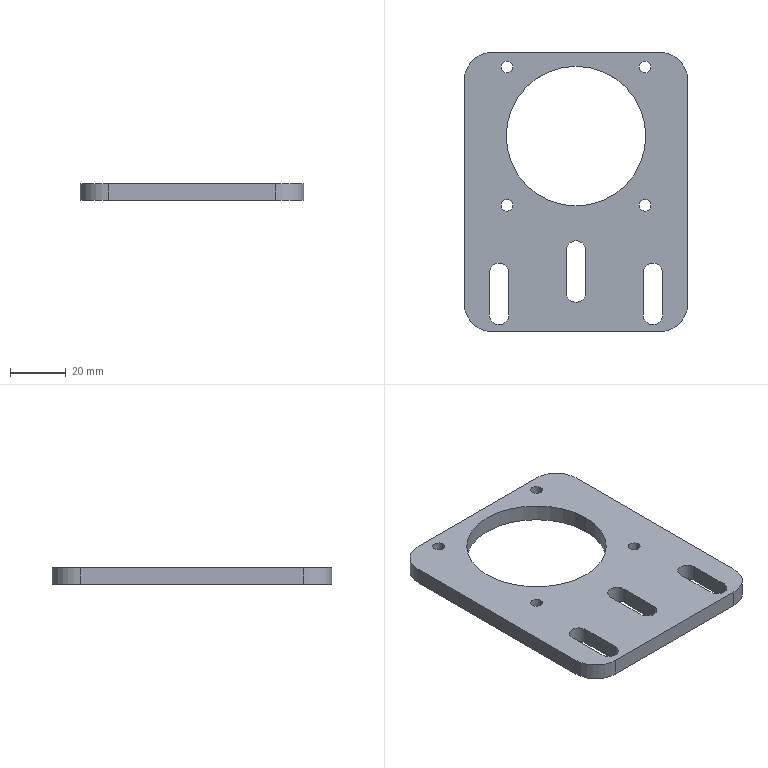Part | STEP file | 1 solid | 32 faces | box 80 x 100 x 6 mm | volume 32789 mm3 | cylinder 20 | plane 12 | commonest cylinder face diameters 4.2 x8 7 x6 20 x4 50 x2